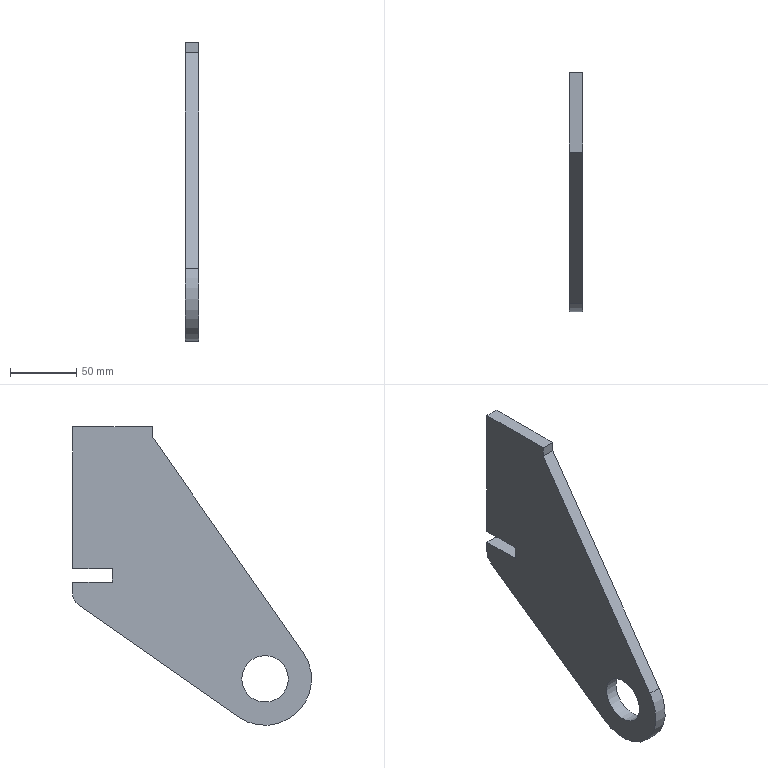Part | STEP file | subframe cylinder mounting plate--000.001--20240928 | 1 solid | 14 faces | box 10 x 180 x 225 mm | volume 214706 mm3 | plane 11 | cylinder 3 | commonest cylinder face diameters 20 x1 35 x1 70 x1
STEP:
#1=CARTESIAN_POINT('',(0.,0.,0.));
#2=DIRECTION('',(0.,0.,1.));
#3=DIRECTION('',(1.,0.,0.));
#4=AXIS2_PLACEMENT_3D('',#1,#2,#3);
#5=CARTESIAN_POINT('',(-10.,145.,64.009));
#6=VERTEX_POINT('',#5);
#7=CARTESIAN_POINT('',(-10.,145.,73.));
#8=VERTEX_POINT('',#7);
#9=CARTESIAN_POINT('',(-10.,145.,-567.));
#10=DIRECTION('',(0.,0.,1.));
#11=VECTOR('',#10,1.);
#12=LINE('',#9,#11);
#13=CARTESIAN_POINT('',(1830.173,145.,190.));
#14=DIRECTION('',(0.,-1.,0.));
#15=DIRECTION('',(1.,0.,0.));
#16=AXIS2_PLACEMENT_3D('',#13,#14,#15);
#17=PLANE('',#16);
#18=CARTESIAN_POINT('',(-1840.173,-757.));
#19=DIRECTION('',(0.,1.));
#20=VECTOR('',#19,1.);
#21=LINE('',#18,#20);
#22=(GEOMETRIC_REPRESENTATION_CONTEXT(2)PARAMETRIC_REPRESENTATION_CONTEXT()REPRESENTATION_CONTEXT('',''));
#23=DEFINITIONAL_REPRESENTATION('',(#21),#22);
#24=PCURVE('',#17,#23);
#25=CARTESIAN_POINT('',(-10.,145.,-567.));
#26=DIRECTION('',(1.,0.,0.));
#27=DIRECTION('',(0.,1.,0.));
#28=AXIS2_PLACEMENT_3D('',#25,#26,#27);
#29=PLANE('',#28);
#30=CARTESIAN_POINT('',(0.,0.));
#31=DIRECTION('',(0.,1.));
#32=VECTOR('',#31,1.);
#33=LINE('',#30,#32);
#34=(GEOMETRIC_REPRESENTATION_CONTEXT(2)PARAMETRIC_REPRESENTATION_CONTEXT()REPRESENTATION_CONTEXT('',''));
#35=DEFINITIONAL_REPRESENTATION('',(#33),#34);
#36=PCURVE('',#29,#35);
#37=SURFACE_CURVE('',#12,(#24,#36),.PCURVE_S1.);
#38=EDGE_CURVE('',#6,#8,#37,.T.);
#39=ORIENTED_EDGE('',*,*,#38,.T.);
#40=CARTESIAN_POINT('',(0.,145.,73.));
#41=VERTEX_POINT('',#40);
#42=CARTESIAN_POINT('',(100.,145.,73.));
#43=DIRECTION('',(1.,0.,0.));
#44=VECTOR('',#43,1.);
#45=LINE('',#42,#44);
#46=CARTESIAN_POINT('',(-1730.173,-117.));
#47=DIRECTION('',(1.,0.));
#48=VECTOR('',#47,1.);
#49=LINE('',#46,#48);
#50=(GEOMETRIC_REPRESENTATION_CONTEXT(2)PARAMETRIC_REPRESENTATION_CONTEXT()REPRESENTATION_CONTEXT('',''));
#51=DEFINITIONAL_REPRESENTATION('',(#49),#50);
#52=PCURVE('',#17,#51);
#53=CARTESIAN_POINT('',(100.,85.,73.));
#54=DIRECTION('',(0.,0.,1.));
#55=DIRECTION('',(0.,-1.,0.));
#56=AXIS2_PLACEMENT_3D('',#53,#54,#55);
#57=PLANE('',#56);
#58=CARTESIAN_POINT('',(-60.,0.));
#59=DIRECTION('',(0.,1.));
#60=VECTOR('',#59,1.);
#61=LINE('',#58,#60);
#62=(GEOMETRIC_REPRESENTATION_CONTEXT(2)PARAMETRIC_REPRESENTATION_CONTEXT()REPRESENTATION_CONTEXT('',''));
#63=DEFINITIONAL_REPRESENTATION('',(#61),#62);
#64=PCURVE('',#57,#63);
#65=SURFACE_CURVE('',#45,(#52,#64),.PCURVE_S1.);
#66=EDGE_CURVE('',#8,#41,#65,.T.);
#67=ORIENTED_EDGE('',*,*,#66,.T.);
#68=CARTESIAN_POINT('',(0.,145.,64.009));
#69=VERTEX_POINT('',#68);
#70=CARTESIAN_POINT('',(0.,145.,-567.));
#71=DIRECTION('',(0.,0.,1.));
#72=VECTOR('',#71,1.);
#73=LINE('',#70,#72);
#74=CARTESIAN_POINT('',(-1830.173,-757.));
#75=DIRECTION('',(0.,1.));
#76=VECTOR('',#75,1.);
#77=LINE('',#74,#76);
#78=(GEOMETRIC_REPRESENTATION_CONTEXT(2)PARAMETRIC_REPRESENTATION_CONTEXT()REPRESENTATION_CONTEXT('',''));
#79=DEFINITIONAL_REPRESENTATION('',(#77),#78);
#80=PCURVE('',#17,#79);
#81=CARTESIAN_POINT('',(0.,145.,-567.));
#82=DIRECTION('',(1.,0.,0.));
#83=DIRECTION('',(0.,1.,0.));
#84=AXIS2_PLACEMENT_3D('',#81,#82,#83);
#85=PLANE('',#84);
#86=CARTESIAN_POINT('',(0.,0.));
#87=DIRECTION('',(0.,1.));
#88=VECTOR('',#87,1.);
#89=LINE('',#86,#88);
#90=(GEOMETRIC_REPRESENTATION_CONTEXT(2)PARAMETRIC_REPRESENTATION_CONTEXT()REPRESENTATION_CONTEXT('',''));
#91=DEFINITIONAL_REPRESENTATION('',(#89),#90);
#92=PCURVE('',#85,#91);
#93=SURFACE_CURVE('',#73,(#80,#92),.PCURVE_S1.);
#94=EDGE_CURVE('',#69,#41,#93,.T.);
#95=ORIENTED_EDGE('',*,*,#94,.F.);
#96=CARTESIAN_POINT('',(1830.173,145.,64.009));
#97=DIRECTION('',(-1.,0.,0.));
#98=VECTOR('',#97,1.);
#99=LINE('',#96,#98);
#100=CARTESIAN_POINT('',(0.,-125.991));
#101=DIRECTION('',(-1.,0.));
#102=VECTOR('',#101,1.);
#103=LINE('',#100,#102);
#104=(GEOMETRIC_REPRESENTATION_CONTEXT(2)PARAMETRIC_REPRESENTATION_CONTEXT()REPRESENTATION_CONTEXT('',''));
#105=DEFINITIONAL_REPRESENTATION('',(#103),#104);
#106=PCURVE('',#17,#105);
#107=CARTESIAN_POINT('',(250.,135.,64.009));
#108=DIRECTION('',(-1.,0.,0.));
#109=DIRECTION('',(0.,1.,0.));
#110=AXIS2_PLACEMENT_3D('',#107,#108,#109);
#111=CYLINDRICAL_SURFACE('',#110,10.);
#112=CARTESIAN_POINT('',(0.,-1580.173));
#113=DIRECTION('',(0.,1.));
#114=VECTOR('',#113,1.);
#115=LINE('',#112,#114);
#116=(GEOMETRIC_REPRESENTATION_CONTEXT(2)PARAMETRIC_REPRESENTATION_CONTEXT()REPRESENTATION_CONTEXT('',''));
#117=DEFINITIONAL_REPRESENTATION('',(#115),#116);
#118=PCURVE('',#111,#117);
#119=SURFACE_CURVE('',#99,(#106,#118),.PCURVE_S1.);
#120=EDGE_CURVE('',#69,#6,#119,.T.);
#121=ORIENTED_EDGE('',*,*,#120,.T.);
#122=EDGE_LOOP('',(#39,#67,#95,#121));
#123=FACE_BOUND('',#122,.T.);
#124=ADVANCED_FACE('',(#123),#17,.F.);
#125=CARTESIAN_POINT('',(-10.,145.,83.));
#126=VERTEX_POINT('',#125);
#127=CARTESIAN_POINT('',(0.,145.,83.));
#128=VERTEX_POINT('',#127);
#129=CARTESIAN_POINT('',(100.,145.,83.));
#130=DIRECTION('',(1.,0.,0.));
#131=VECTOR('',#130,1.);
#132=LINE('',#129,#131);
#133=CARTESIAN_POINT('',(1830.173,145.,190.));
#134=DIRECTION('',(0.,-1.,0.));
#135=DIRECTION('',(1.,0.,0.));
#136=AXIS2_PLACEMENT_3D('',#133,#134,#135);
#137=PLANE('',#136);
#138=CARTESIAN_POINT('',(-1730.173,-107.));
#139=DIRECTION('',(1.,0.));
#140=VECTOR('',#139,1.);
#141=LINE('',#138,#140);
#142=(GEOMETRIC_REPRESENTATION_CONTEXT(2)PARAMETRIC_REPRESENTATION_CONTEXT()REPRESENTATION_CONTEXT('',''));
#143=DEFINITIONAL_REPRESENTATION('',(#141),#142);
#144=PCURVE('',#137,#143);
#145=CARTESIAN_POINT('',(100.,85.,83.));
#146=DIRECTION('',(0.,0.,1.));
#147=DIRECTION('',(0.,-1.,0.));
#148=AXIS2_PLACEMENT_3D('',#145,#146,#147);
#149=PLANE('',#148);
#150=CARTESIAN_POINT('',(-60.,0.));
#151=DIRECTION('',(0.,1.));
#152=VECTOR('',#151,1.);
#153=LINE('',#150,#152);
#154=(GEOMETRIC_REPRESENTATION_CONTEXT(2)PARAMETRIC_REPRESENTATION_CONTEXT()REPRESENTATION_CONTEXT('',''));
#155=DEFINITIONAL_REPRESENTATION('',(#153),#154);
#156=PCURVE('',#149,#155);
#157=SURFACE_CURVE('',#132,(#144,#156),.PCURVE_S1.);
#158=EDGE_CURVE('',#126,#128,#157,.T.);
#159=ORIENTED_EDGE('',*,*,#158,.F.);
#160=CARTESIAN_POINT('',(-10.,145.,190.));
#161=VERTEX_POINT('',#160);
#162=CARTESIAN_POINT('',(-10.,145.,-567.));
#163=DIRECTION('',(0.,0.,1.));
#164=VECTOR('',#163,1.);
#165=LINE('',#162,#164);
#166=CARTESIAN_POINT('',(-1840.173,-757.));
#167=DIRECTION('',(0.,1.));
#168=VECTOR('',#167,1.);
#169=LINE('',#166,#168);
#170=(GEOMETRIC_REPRESENTATION_CONTEXT(2)PARAMETRIC_REPRESENTATION_CONTEXT()REPRESENTATION_CONTEXT('',''));
#171=DEFINITIONAL_REPRESENTATION('',(#169),#170);
#172=PCURVE('',#137,#171);
#173=CARTESIAN_POINT('',(0.,0.));
#174=DIRECTION('',(0.,1.));
#175=VECTOR('',#174,1.);
#176=LINE('',#173,#175);
#177=(GEOMETRIC_REPRESENTATION_CONTEXT(2)PARAMETRIC_REPRESENTATION_CONTEXT()REPRESENTATION_CONTEXT('',''));
#178=DEFINITIONAL_REPRESENTATION('',(#176),#177);
#179=PCURVE('',#29,#178);
#180=SURFACE_CURVE('',#165,(#172,#179),.PCURVE_S1.);
#181=EDGE_CURVE('',#126,#161,#180,.T.);
#182=ORIENTED_EDGE('',*,*,#181,.T.);
#183=CARTESIAN_POINT('',(0.,145.,190.));
#184=VERTEX_POINT('',#183);
#185=CARTESIAN_POINT('',(1830.173,145.,190.));
#186=DIRECTION('',(1.,0.,0.));
#187=VECTOR('',#186,1.);
#188=LINE('',#185,#187);
#189=CARTESIAN_POINT('',(0.,0.));
#190=DIRECTION('',(1.,0.));
#191=VECTOR('',#190,1.);
#192=LINE('',#189,#191);
#193=(GEOMETRIC_REPRESENTATION_CONTEXT(2)PARAMETRIC_REPRESENTATION_CONTEXT()REPRESENTATION_CONTEXT('',''));
#194=DEFINITIONAL_REPRESENTATION('',(#192),#193);
#195=PCURVE('',#137,#194);
#196=CARTESIAN_POINT('',(250.,115.,190.));
#197=DIRECTION('',(0.,0.,1.));
#198=DIRECTION('',(-0.2756,0.9613,0.));
#199=AXIS2_PLACEMENT_3D('',#196,#197,#198);
#200=PLANE('',#199);
#201=CARTESIAN_POINT('',(-406.717,-1527.229));
#202=DIRECTION('',(-0.2756,-0.9613));
#203=VECTOR('',#202,1.);
#204=LINE('',#201,#203);
#205=(GEOMETRIC_REPRESENTATION_CONTEXT(2)PARAMETRIC_REPRESENTATION_CONTEXT()REPRESENTATION_CONTEXT('',''));
#206=DEFINITIONAL_REPRESENTATION('',(#204),#205);
#207=PCURVE('',#200,#206);
#208=SURFACE_CURVE('',#188,(#195,#207),.PCURVE_S1.);
#209=EDGE_CURVE('',#161,#184,#208,.T.);
#210=ORIENTED_EDGE('',*,*,#209,.T.);
#211=CARTESIAN_POINT('',(0.,145.,-567.));
#212=DIRECTION('',(0.,0.,1.));
#213=VECTOR('',#212,1.);
#214=LINE('',#211,#213);
#215=CARTESIAN_POINT('',(-1830.173,-757.));
#216=DIRECTION('',(0.,1.));
#217=VECTOR('',#216,1.);
#218=LINE('',#215,#217);
#219=(GEOMETRIC_REPRESENTATION_CONTEXT(2)PARAMETRIC_REPRESENTATION_CONTEXT()REPRESENTATION_CONTEXT('',''));
#220=DEFINITIONAL_REPRESENTATION('',(#218),#219);
#221=PCURVE('',#137,#220);
#222=CARTESIAN_POINT('',(0.,0.));
#223=DIRECTION('',(0.,1.));
#224=VECTOR('',#223,1.);
#225=LINE('',#222,#224);
#226=(GEOMETRIC_REPRESENTATION_CONTEXT(2)PARAMETRIC_REPRESENTATION_CONTEXT()REPRESENTATION_CONTEXT('',''));
#227=DEFINITIONAL_REPRESENTATION('',(#225),#226);
#228=PCURVE('',#85,#227);
#229=SURFACE_CURVE('',#214,(#221,#228),.PCURVE_S1.);
#230=EDGE_CURVE('',#128,#184,#229,.T.);
#231=ORIENTED_EDGE('',*,*,#230,.F.);
#232=EDGE_LOOP('',(#159,#182,#210,#231));
#233=FACE_BOUND('',#232,.T.);
#234=ADVANCED_FACE('',(#233),#137,.F.);
#235=CARTESIAN_POINT('',(-10.,115.,83.));
#236=VERTEX_POINT('',#235);
#237=CARTESIAN_POINT('',(-10.,145.,83.));
#238=DIRECTION('',(0.,-1.,0.));
#239=VECTOR('',#238,1.);
#240=LINE('',#237,#239);
#241=CARTESIAN_POINT('',(0.,650.));
#242=DIRECTION('',(-1.,0.));
#243=VECTOR('',#242,1.);
#244=LINE('',#241,#243);
#245=(GEOMETRIC_REPRESENTATION_CONTEXT(2)PARAMETRIC_REPRESENTATION_CONTEXT()REPRESENTATION_CONTEXT('',''));
#246=DEFINITIONAL_REPRESENTATION('',(#244),#245);
#247=PCURVE('',#29,#246);
#248=CARTESIAN_POINT('',(-60.,-110.));
#249=DIRECTION('',(1.,0.));
#250=VECTOR('',#249,1.);
#251=LINE('',#248,#250);
#252=(GEOMETRIC_REPRESENTATION_CONTEXT(2)PARAMETRIC_REPRESENTATION_CONTEXT()REPRESENTATION_CONTEXT('',''));
#253=DEFINITIONAL_REPRESENTATION('',(#251),#252);
#254=PCURVE('',#149,#253);
#255=SURFACE_CURVE('',#240,(#247,#254),.PCURVE_S1.);
#256=EDGE_CURVE('',#126,#236,#255,.T.);
#257=ORIENTED_EDGE('',*,*,#256,.T.);
#258=CARTESIAN_POINT('',(-10.,115.,73.));
#259=VERTEX_POINT('',#258);
#260=CARTESIAN_POINT('',(-10.,115.,78.));
#261=DIRECTION('',(0.,0.,-1.));
#262=VECTOR('',#261,1.);
#263=LINE('',#260,#262);
#264=CARTESIAN_POINT('',(-30.,645.));
#265=DIRECTION('',(0.,-1.));
#266=VECTOR('',#265,1.);
#267=LINE('',#264,#266);
#268=(GEOMETRIC_REPRESENTATION_CONTEXT(2)PARAMETRIC_REPRESENTATION_CONTEXT()REPRESENTATION_CONTEXT('',''));
#269=DEFINITIONAL_REPRESENTATION('',(#267),#268);
#270=PCURVE('',#29,#269);
#271=CARTESIAN_POINT('',(95.,115.,78.));
#272=DIRECTION('',(0.,1.,0.));
#273=DIRECTION('',(1.,0.,0.));
#274=AXIS2_PLACEMENT_3D('',#271,#272,#273);
#275=PLANE('',#274);
#276=CARTESIAN_POINT('',(-105.,0.));
#277=DIRECTION('',(0.,1.));
#278=VECTOR('',#277,1.);
#279=LINE('',#276,#278);
#280=(GEOMETRIC_REPRESENTATION_CONTEXT(2)PARAMETRIC_REPRESENTATION_CONTEXT()REPRESENTATION_CONTEXT('',''));
#281=DEFINITIONAL_REPRESENTATION('',(#279),#280);
#282=PCURVE('',#275,#281);
#283=SURFACE_CURVE('',#263,(#270,#282),.PCURVE_S1.);
#284=EDGE_CURVE('',#236,#259,#283,.T.);
#285=ORIENTED_EDGE('',*,*,#284,.T.);
#286=CARTESIAN_POINT('',(-10.,145.,73.));
#287=DIRECTION('',(0.,1.,0.));
#288=VECTOR('',#287,1.);
#289=LINE('',#286,#288);
#290=CARTESIAN_POINT('',(0.,640.));
#291=DIRECTION('',(1.,0.));
#292=VECTOR('',#291,1.);
#293=LINE('',#290,#292);
#294=(GEOMETRIC_REPRESENTATION_CONTEXT(2)PARAMETRIC_REPRESENTATION_CONTEXT()REPRESENTATION_CONTEXT('',''));
#295=DEFINITIONAL_REPRESENTATION('',(#293),#294);
#296=PCURVE('',#29,#295);
#297=CARTESIAN_POINT('',(-60.,-110.));
#298=DIRECTION('',(-1.,0.));
#299=VECTOR('',#298,1.);
#300=LINE('',#297,#299);
#301=(GEOMETRIC_REPRESENTATION_CONTEXT(2)PARAMETRIC_REPRESENTATION_CONTEXT()REPRESENTATION_CONTEXT('',''));
#302=DEFINITIONAL_REPRESENTATION('',(#300),#301);
#303=PCURVE('',#57,#302);
#304=SURFACE_CURVE('',#289,(#296,#303),.PCURVE_S1.);
#305=EDGE_CURVE('',#259,#8,#304,.T.);
#306=ORIENTED_EDGE('',*,*,#305,.T.);
#307=ORIENTED_EDGE('',*,*,#38,.F.);
#308=CARTESIAN_POINT('',(-10.,140.736,55.817));
#309=VERTEX_POINT('',#308);
#310=CARTESIAN_POINT('',(-10.,135.,64.009));
#311=DIRECTION('',(-1.,0.,0.));
#312=DIRECTION('',(0.,0.,-1.));
#313=AXIS2_PLACEMENT_3D('',#310,#311,#312);
#314=CIRCLE('',#313,10.);
#315=CARTESIAN_POINT('',(-10.,621.009));
#316=CARTESIAN_POINT('',(-27.321,621.009));
#317=CARTESIAN_POINT('',(-18.66,636.009));
#318=CARTESIAN_POINT('',(-10.,651.009));
#319=CARTESIAN_POINT('',(-1.34,636.009));
#320=CARTESIAN_POINT('',(7.321,621.009));
#321=CARTESIAN_POINT('',(-10.,621.009));
#322=(BOUNDED_CURVE()B_SPLINE_CURVE(2,(#315,#316,#317,#318,#319,#320,#321),.UNSPECIFIED.,.T.,.F.)B_SPLINE_CURVE_WITH_KNOTS((1,2,2,2,2,1),(-2.094,0.,2.094,4.189,6.283,8.378),.UNSPECIFIED.)CURVE()GEOMETRIC_REPRESENTATION_ITEM()RATIONAL_B_SPLINE_CURVE((1.,0.5,1.,0.5,1.,0.5,1.))REPRESENTATION_ITEM(''));
#323=(GEOMETRIC_REPRESENTATION_CONTEXT(2)PARAMETRIC_REPRESENTATION_CONTEXT()REPRESENTATION_CONTEXT('',''));
#324=DEFINITIONAL_REPRESENTATION('',(#322),#323);
#325=PCURVE('',#29,#324);
#326=CARTESIAN_POINT('',(-4.712,260.));
#327=DIRECTION('',(1.,0.));
#328=VECTOR('',#327,1.);
#329=LINE('',#326,#328);
#330=(GEOMETRIC_REPRESENTATION_CONTEXT(2)PARAMETRIC_REPRESENTATION_CONTEXT()REPRESENTATION_CONTEXT('',''));
#331=DEFINITIONAL_REPRESENTATION('',(#329),#330);
#332=PCURVE('',#111,#331);
#333=SURFACE_CURVE('',#314,(#325,#332),.PCURVE_S1.);
#334=EDGE_CURVE('',#6,#309,#333,.T.);
#335=ORIENTED_EDGE('',*,*,#334,.T.);
#336=CARTESIAN_POINT('',(-10.,20.075,-28.67));
#337=VERTEX_POINT('',#336);
#338=CARTESIAN_POINT('',(-10.,-149.031,-147.08));
#339=DIRECTION('',(0.,-0.8192,-0.5736));
#340=VECTOR('',#339,1.);
#341=LINE('',#338,#340);
#342=CARTESIAN_POINT('',(-294.031,419.92));
#343=DIRECTION('',(-0.8192,-0.5736));
#344=VECTOR('',#343,1.);
#345=LINE('',#342,#344);
#346=(GEOMETRIC_REPRESENTATION_CONTEXT(2)PARAMETRIC_REPRESENTATION_CONTEXT()REPRESENTATION_CONTEXT('',''));
#347=DEFINITIONAL_REPRESENTATION('',(#345),#346);
#348=PCURVE('',#29,#347);
#349=CARTESIAN_POINT('',(250.,114.278,37.291));
#350=DIRECTION('',(0.,0.5736,-0.8192));
#351=DIRECTION('',(0.2756,-0.7874,-0.5514));
#352=AXIS2_PLACEMENT_3D('',#349,#350,#351);
#353=PLANE('',#352);
#354=CARTESIAN_POINT('',(237.323,338.529));
#355=DIRECTION('',(0.9613,0.2756));
#356=VECTOR('',#355,1.);
#357=LINE('',#354,#356);
#358=(GEOMETRIC_REPRESENTATION_CONTEXT(2)PARAMETRIC_REPRESENTATION_CONTEXT()REPRESENTATION_CONTEXT('',''));
#359=DEFINITIONAL_REPRESENTATION('',(#357),#358);
#360=PCURVE('',#353,#359);
#361=SURFACE_CURVE('',#341,(#348,#360),.PCURVE_S1.);
#362=EDGE_CURVE('',#309,#337,#361,.T.);
#363=ORIENTED_EDGE('',*,*,#362,.T.);
#364=CARTESIAN_POINT('',(-10.,-28.67,20.075));
#365=VERTEX_POINT('',#364);
#366=CARTESIAN_POINT('',(-10.,0.,0.));
#367=DIRECTION('',(-1.,0.,0.));
#368=DIRECTION('',(0.,0.,-1.));
#369=AXIS2_PLACEMENT_3D('',#366,#367,#368);
#370=CIRCLE('',#369,35.);
#371=CARTESIAN_POINT('',(-145.,532.));
#372=CARTESIAN_POINT('',(-205.622,532.));
#373=CARTESIAN_POINT('',(-175.311,584.5));
#374=CARTESIAN_POINT('',(-145.,637.));
#375=CARTESIAN_POINT('',(-114.689,584.5));
#376=CARTESIAN_POINT('',(-84.378,532.));
#377=CARTESIAN_POINT('',(-145.,532.));
#378=(BOUNDED_CURVE()B_SPLINE_CURVE(2,(#371,#372,#373,#374,#375,#376,#377),.UNSPECIFIED.,.T.,.F.)B_SPLINE_CURVE_WITH_KNOTS((1,2,2,2,2,1),(-2.094,0.,2.094,4.189,6.283,8.378),.UNSPECIFIED.)CURVE()GEOMETRIC_REPRESENTATION_ITEM()RATIONAL_B_SPLINE_CURVE((1.,0.5,1.,0.5,1.,0.5,1.))REPRESENTATION_ITEM(''));
#379=(GEOMETRIC_REPRESENTATION_CONTEXT(2)PARAMETRIC_REPRESENTATION_CONTEXT()REPRESENTATION_CONTEXT('',''));
#380=DEFINITIONAL_REPRESENTATION('',(#378),#379);
#381=PCURVE('',#29,#380);
#382=CARTESIAN_POINT('',(-30.,0.,0.));
#383=DIRECTION('',(1.,0.,0.));
#384=DIRECTION('',(0.,0.,1.));
#385=AXIS2_PLACEMENT_3D('',#382,#383,#384);
#386=CYLINDRICAL_SURFACE('',#385,35.);
#387=CARTESIAN_POINT('',(9.425,20.));
#388=DIRECTION('',(-1.,0.));
#389=VECTOR('',#388,1.);
#390=LINE('',#387,#389);
#391=(GEOMETRIC_REPRESENTATION_CONTEXT(2)PARAMETRIC_REPRESENTATION_CONTEXT()REPRESENTATION_CONTEXT('',''));
#392=DEFINITIONAL_REPRESENTATION('',(#390),#391);
#393=PCURVE('',#386,#392);
#394=SURFACE_CURVE('',#370,(#381,#393),.PCURVE_S1.);
#395=EDGE_CURVE('',#337,#365,#394,.T.);
#396=ORIENTED_EDGE('',*,*,#395,.T.);
#397=CARTESIAN_POINT('',(-10.,85.,182.413));
#398=VERTEX_POINT('',#397);
#399=CARTESIAN_POINT('',(-10.,-25.831,24.13));
#400=DIRECTION('',(0.,0.5736,0.8192));
#401=VECTOR('',#400,1.);
#402=LINE('',#399,#401);
#403=CARTESIAN_POINT('',(-170.831,591.13));
#404=DIRECTION('',(0.5736,0.8192));
#405=VECTOR('',#404,1.);
#406=LINE('',#403,#405);
#407=(GEOMETRIC_REPRESENTATION_CONTEXT(2)PARAMETRIC_REPRESENTATION_CONTEXT()REPRESENTATION_CONTEXT('',''));
#408=DEFINITIONAL_REPRESENTATION('',(#406),#407);
#409=PCURVE('',#29,#408);
#410=CARTESIAN_POINT('',(-30.,-25.831,24.13));
#411=DIRECTION('',(0.,-0.8192,0.5736));
#412=DIRECTION('',(-1.,0.,0.));
#413=AXIS2_PLACEMENT_3D('',#410,#411,#412);
#414=PLANE('',#413);
#415=CARTESIAN_POINT('',(-20.,0.));
#416=DIRECTION('',(0.,-1.));
#417=VECTOR('',#416,1.);
#418=LINE('',#415,#417);
#419=(GEOMETRIC_REPRESENTATION_CONTEXT(2)PARAMETRIC_REPRESENTATION_CONTEXT()REPRESENTATION_CONTEXT('',''));
#420=DEFINITIONAL_REPRESENTATION('',(#418),#419);
#421=PCURVE('',#414,#420);
#422=SURFACE_CURVE('',#402,(#409,#421),.PCURVE_S1.);
#423=EDGE_CURVE('',#365,#398,#422,.T.);
#424=ORIENTED_EDGE('',*,*,#423,.T.);
#425=CARTESIAN_POINT('',(-10.,85.,190.));
#426=VERTEX_POINT('',#425);
#427=CARTESIAN_POINT('',(-10.,85.,-567.));
#428=DIRECTION('',(0.,0.,1.));
#429=VECTOR('',#428,1.);
#430=LINE('',#427,#429);
#431=CARTESIAN_POINT('',(-60.,0.));
#432=DIRECTION('',(0.,1.));
#433=VECTOR('',#432,1.);
#434=LINE('',#431,#433);
#435=(GEOMETRIC_REPRESENTATION_CONTEXT(2)PARAMETRIC_REPRESENTATION_CONTEXT()REPRESENTATION_CONTEXT('',''));
#436=DEFINITIONAL_REPRESENTATION('',(#434),#435);
#437=PCURVE('',#29,#436);
#438=CARTESIAN_POINT('',(-5.,85.,210.));
#439=DIRECTION('',(0.,1.,0.));
#440=DIRECTION('',(0.,0.,-1.));
#441=AXIS2_PLACEMENT_3D('',#438,#439,#440);
#442=PLANE('',#441);
#443=CARTESIAN_POINT('',(777.,5.));
#444=DIRECTION('',(-1.,0.));
#445=VECTOR('',#444,1.);
#446=LINE('',#443,#445);
#447=(GEOMETRIC_REPRESENTATION_CONTEXT(2)PARAMETRIC_REPRESENTATION_CONTEXT()REPRESENTATION_CONTEXT('',''));
#448=DEFINITIONAL_REPRESENTATION('',(#446),#447);
#449=PCURVE('',#442,#448);
#450=SURFACE_CURVE('',#430,(#437,#449),.PCURVE_S1.);
#451=EDGE_CURVE('',#398,#426,#450,.T.);
#452=ORIENTED_EDGE('',*,*,#451,.T.);
#453=CARTESIAN_POINT('',(-10.,145.,190.));
#454=DIRECTION('',(0.,-1.,0.));
#455=VECTOR('',#454,1.);
#456=LINE('',#453,#455);
#457=CARTESIAN_POINT('',(0.,757.));
#458=DIRECTION('',(-1.,0.));
#459=VECTOR('',#458,1.);
#460=LINE('',#457,#459);
#461=(GEOMETRIC_REPRESENTATION_CONTEXT(2)PARAMETRIC_REPRESENTATION_CONTEXT()REPRESENTATION_CONTEXT('',''));
#462=DEFINITIONAL_REPRESENTATION('',(#460),#461);
#463=PCURVE('',#29,#462);
#464=CARTESIAN_POINT('',(100.504,241.659));
#465=DIRECTION('',(-0.9613,0.2756));
#466=VECTOR('',#465,1.);
#467=LINE('',#464,#466);
#468=(GEOMETRIC_REPRESENTATION_CONTEXT(2)PARAMETRIC_REPRESENTATION_CONTEXT()REPRESENTATION_CONTEXT('',''));
#469=DEFINITIONAL_REPRESENTATION('',(#467),#468);
#470=PCURVE('',#200,#469);
#471=SURFACE_CURVE('',#456,(#463,#470),.PCURVE_S1.);
#472=EDGE_CURVE('',#161,#426,#471,.T.);
#473=ORIENTED_EDGE('',*,*,#472,.F.);
#474=ORIENTED_EDGE('',*,*,#181,.F.);
#475=EDGE_LOOP('',(#257,#285,#306,#307,#335,#363,#396,#424,#452,#473,#474));
#476=FACE_BOUND('',#475,.T.);
#477=CARTESIAN_POINT('',(-10.,-17.5,0.));
#478=VERTEX_POINT('',#477);
#479=CARTESIAN_POINT('',(-10.,0.,0.));
#480=DIRECTION('',(1.,0.,0.));
#481=DIRECTION('',(0.,-1.,0.));
#482=AXIS2_PLACEMENT_3D('',#479,#480,#481);
#483=CIRCLE('',#482,17.5);
#484=CARTESIAN_POINT('',(-145.,567.));
#485=DIRECTION('',(-1.,0.));
#486=AXIS2_PLACEMENT_2D('',#484,#485);
#487=CIRCLE('',#486,17.5);
#488=(GEOMETRIC_REPRESENTATION_CONTEXT(2)PARAMETRIC_REPRESENTATION_CONTEXT()REPRESENTATION_CONTEXT('',''));
#489=DEFINITIONAL_REPRESENTATION('',(#487),#488);
#490=PCURVE('',#29,#489);
#491=CARTESIAN_POINT('',(-360.,0.,0.));
#492=DIRECTION('',(1.,0.,0.));
#493=DIRECTION('',(0.,1.,0.));
#494=AXIS2_PLACEMENT_3D('',#491,#492,#493);
#495=CYLINDRICAL_SURFACE('',#494,17.5);
#496=CARTESIAN_POINT('',(3.142,350.));
#497=DIRECTION('',(1.,0.));
#498=VECTOR('',#497,1.);
#499=LINE('',#496,#498);
#500=(GEOMETRIC_REPRESENTATION_CONTEXT(2)PARAMETRIC_REPRESENTATION_CONTEXT()REPRESENTATION_CONTEXT('',''));
#501=DEFINITIONAL_REPRESENTATION('',(#499),#500);
#502=PCURVE('',#495,#501);
#503=SURFACE_CURVE('',#483,(#490,#502),.PCURVE_S1.);
#504=EDGE_CURVE('',#478,#478,#503,.T.);
#505=ORIENTED_EDGE('',*,*,#504,.T.);
#506=EDGE_LOOP('',(#505));
#507=FACE_BOUND('',#506,.T.);
#508=ADVANCED_FACE('',(#476,#507),#29,.F.);
#509=CARTESIAN_POINT('',(0.,115.,83.));
#510=VERTEX_POINT('',#509);
#511=CARTESIAN_POINT('',(0.,115.,73.));
#512=VERTEX_POINT('',#511);
#513=CARTESIAN_POINT('',(0.,115.,78.));
#514=DIRECTION('',(0.,0.,-1.));
#515=VECTOR('',#514,1.);
#516=LINE('',#513,#515);
#517=CARTESIAN_POINT('',(-30.,645.));
#518=DIRECTION('',(0.,-1.));
#519=VECTOR('',#518,1.);
#520=LINE('',#517,#519);
#521=(GEOMETRIC_REPRESENTATION_CONTEXT(2)PARAMETRIC_REPRESENTATION_CONTEXT()REPRESENTATION_CONTEXT('',''));
#522=DEFINITIONAL_REPRESENTATION('',(#520),#521);
#523=PCURVE('',#85,#522);
#524=CARTESIAN_POINT('',(-95.,0.));
#525=DIRECTION('',(0.,1.));
#526=VECTOR('',#525,1.);
#527=LINE('',#524,#526);
#528=(GEOMETRIC_REPRESENTATION_CONTEXT(2)PARAMETRIC_REPRESENTATION_CONTEXT()REPRESENTATION_CONTEXT('',''));
#529=DEFINITIONAL_REPRESENTATION('',(#527),#528);
#530=PCURVE('',#275,#529);
#531=SURFACE_CURVE('',#516,(#523,#530),.PCURVE_S1.);
#532=EDGE_CURVE('',#510,#512,#531,.T.);
#533=ORIENTED_EDGE('',*,*,#532,.F.);
#534=CARTESIAN_POINT('',(0.,145.,83.));
#535=DIRECTION('',(0.,-1.,0.));
#536=VECTOR('',#535,1.);
#537=LINE('',#534,#536);
#538=CARTESIAN_POINT('',(0.,650.));
#539=DIRECTION('',(-1.,0.));
#540=VECTOR('',#539,1.);
#541=LINE('',#538,#540);
#542=(GEOMETRIC_REPRESENTATION_CONTEXT(2)PARAMETRIC_REPRESENTATION_CONTEXT()REPRESENTATION_CONTEXT('',''));
#543=DEFINITIONAL_REPRESENTATION('',(#541),#542);
#544=PCURVE('',#85,#543);
#545=CARTESIAN_POINT('',(-60.,-100.));
#546=DIRECTION('',(1.,0.));
#547=VECTOR('',#546,1.);
#548=LINE('',#545,#547);
#549=(GEOMETRIC_REPRESENTATION_CONTEXT(2)PARAMETRIC_REPRESENTATION_CONTEXT()REPRESENTATION_CONTEXT('',''));
#550=DEFINITIONAL_REPRESENTATION('',(#548),#549);
#551=PCURVE('',#149,#550);
#552=SURFACE_CURVE('',#537,(#544,#551),.PCURVE_S1.);
#553=EDGE_CURVE('',#128,#510,#552,.T.);
#554=ORIENTED_EDGE('',*,*,#553,.F.);
#555=ORIENTED_EDGE('',*,*,#230,.T.);
#556=CARTESIAN_POINT('',(0.,85.,190.));
#557=VERTEX_POINT('',#556);
#558=CARTESIAN_POINT('',(0.,145.,190.));
#559=DIRECTION('',(0.,-1.,0.));
#560=VECTOR('',#559,1.);
#561=LINE('',#558,#560);
#562=CARTESIAN_POINT('',(0.,757.));
#563=DIRECTION('',(-1.,0.));
#564=VECTOR('',#563,1.);
#565=LINE('',#562,#564);
#566=(GEOMETRIC_REPRESENTATION_CONTEXT(2)PARAMETRIC_REPRESENTATION_CONTEXT()REPRESENTATION_CONTEXT('',''));
#567=DEFINITIONAL_REPRESENTATION('',(#565),#566);
#568=PCURVE('',#85,#567);
#569=CARTESIAN_POINT('',(97.747,232.046));
#570=DIRECTION('',(-0.9613,0.2756));
#571=VECTOR('',#570,1.);
#572=LINE('',#569,#571);
#573=(GEOMETRIC_REPRESENTATION_CONTEXT(2)PARAMETRIC_REPRESENTATION_CONTEXT()REPRESENTATION_CONTEXT('',''));
#574=DEFINITIONAL_REPRESENTATION('',(#572),#573);
#575=PCURVE('',#200,#574);
#576=SURFACE_CURVE('',#561,(#568,#575),.PCURVE_S1.);
#577=EDGE_CURVE('',#184,#557,#576,.T.);
#578=ORIENTED_EDGE('',*,*,#577,.T.);
#579=CARTESIAN_POINT('',(0.,85.,182.413));
#580=VERTEX_POINT('',#579);
#581=CARTESIAN_POINT('',(0.,85.,-567.));
#582=DIRECTION('',(0.,0.,1.));
#583=VECTOR('',#582,1.);
#584=LINE('',#581,#583);
#585=CARTESIAN_POINT('',(-60.,0.));
#586=DIRECTION('',(0.,1.));
#587=VECTOR('',#586,1.);
#588=LINE('',#585,#587);
#589=(GEOMETRIC_REPRESENTATION_CONTEXT(2)PARAMETRIC_REPRESENTATION_CONTEXT()REPRESENTATION_CONTEXT('',''));
#590=DEFINITIONAL_REPRESENTATION('',(#588),#589);
#591=PCURVE('',#85,#590);
#592=CARTESIAN_POINT('',(777.,-5.));
#593=DIRECTION('',(-1.,0.));
#594=VECTOR('',#593,1.);
#595=LINE('',#592,#594);
#596=(GEOMETRIC_REPRESENTATION_CONTEXT(2)PARAMETRIC_REPRESENTATION_CONTEXT()REPRESENTATION_CONTEXT('',''));
#597=DEFINITIONAL_REPRESENTATION('',(#595),#596);
#598=PCURVE('',#442,#597);
#599=SURFACE_CURVE('',#584,(#591,#598),.PCURVE_S1.);
#600=EDGE_CURVE('',#580,#557,#599,.T.);
#601=ORIENTED_EDGE('',*,*,#600,.F.);
#602=CARTESIAN_POINT('',(0.,-28.67,20.075));
#603=VERTEX_POINT('',#602);
#604=CARTESIAN_POINT('',(0.,-247.37,-292.26));
#605=DIRECTION('',(0.,-0.5736,-0.8192));
#606=VECTOR('',#605,1.);
#607=LINE('',#604,#606);
#608=CARTESIAN_POINT('',(-392.37,274.74));
#609=DIRECTION('',(-0.5736,-0.8192));
#610=VECTOR('',#609,1.);
#611=LINE('',#608,#610);
#612=(GEOMETRIC_REPRESENTATION_CONTEXT(2)PARAMETRIC_REPRESENTATION_CONTEXT()REPRESENTATION_CONTEXT('',''));
#613=DEFINITIONAL_REPRESENTATION('',(#611),#612);
#614=PCURVE('',#85,#613);
#615=CARTESIAN_POINT('',(-30.,386.24));
#616=DIRECTION('',(0.,1.));
#617=VECTOR('',#616,1.);
#618=LINE('',#615,#617);
#619=(GEOMETRIC_REPRESENTATION_CONTEXT(2)PARAMETRIC_REPRESENTATION_CONTEXT()REPRESENTATION_CONTEXT('',''));
#620=DEFINITIONAL_REPRESENTATION('',(#618),#619);
#621=PCURVE('',#414,#620);
#622=SURFACE_CURVE('',#607,(#614,#621),.PCURVE_S1.);
#623=EDGE_CURVE('',#580,#603,#622,.T.);
#624=ORIENTED_EDGE('',*,*,#623,.T.);
#625=CARTESIAN_POINT('',(0.,20.075,-28.67));
#626=VERTEX_POINT('',#625);
#627=CARTESIAN_POINT('',(0.,0.,0.));
#628=DIRECTION('',(1.,0.,0.));
#629=DIRECTION('',(0.,0.,-1.));
#630=AXIS2_PLACEMENT_3D('',#627,#628,#629);
#631=CIRCLE('',#630,35.);
#632=CARTESIAN_POINT('',(-145.,567.));
#633=DIRECTION('',(0.,-1.));
#634=AXIS2_PLACEMENT_2D('',#632,#633);
#635=CIRCLE('',#634,35.);
#636=(GEOMETRIC_REPRESENTATION_CONTEXT(2)PARAMETRIC_REPRESENTATION_CONTEXT()REPRESENTATION_CONTEXT('',''));
#637=DEFINITIONAL_REPRESENTATION('',(#635),#636);
#638=PCURVE('',#85,#637);
#639=CARTESIAN_POINT('',(-3.142,30.));
#640=DIRECTION('',(1.,0.));
#641=VECTOR('',#640,1.);
#642=LINE('',#639,#641);
#643=(GEOMETRIC_REPRESENTATION_CONTEXT(2)PARAMETRIC_REPRESENTATION_CONTEXT()REPRESENTATION_CONTEXT('',''));
#644=DEFINITIONAL_REPRESENTATION('',(#642),#643);
#645=PCURVE('',#386,#644);
#646=SURFACE_CURVE('',#631,(#638,#645),.PCURVE_S1.);
#647=EDGE_CURVE('',#603,#626,#646,.T.);
#648=ORIENTED_EDGE('',*,*,#647,.T.);
#649=CARTESIAN_POINT('',(0.,140.736,55.817));
#650=VERTEX_POINT('',#649);
#651=CARTESIAN_POINT('',(0.,-149.031,-147.08));
#652=DIRECTION('',(0.,-0.8192,-0.5736));
#653=VECTOR('',#652,1.);
#654=LINE('',#651,#653);
#655=CARTESIAN_POINT('',(-294.031,419.92));
#656=DIRECTION('',(-0.8192,-0.5736));
#657=VECTOR('',#656,1.);
#658=LINE('',#655,#657);
#659=(GEOMETRIC_REPRESENTATION_CONTEXT(2)PARAMETRIC_REPRESENTATION_CONTEXT()REPRESENTATION_CONTEXT('',''));
#660=DEFINITIONAL_REPRESENTATION('',(#658),#659);
#661=PCURVE('',#85,#660);
#662=CARTESIAN_POINT('',(240.079,328.917));
#663=DIRECTION('',(0.9613,0.2756));
#664=VECTOR('',#663,1.);
#665=LINE('',#662,#664);
#666=(GEOMETRIC_REPRESENTATION_CONTEXT(2)PARAMETRIC_REPRESENTATION_CONTEXT()REPRESENTATION_CONTEXT('',''));
#667=DEFINITIONAL_REPRESENTATION('',(#665),#666);
#668=PCURVE('',#353,#667);
#669=SURFACE_CURVE('',#654,(#661,#668),.PCURVE_S1.);
#670=EDGE_CURVE('',#650,#626,#669,.T.);
#671=ORIENTED_EDGE('',*,*,#670,.F.);
#672=CARTESIAN_POINT('',(0.,135.,64.009));
#673=DIRECTION('',(1.,0.,0.));
#674=DIRECTION('',(0.,0.,-1.));
#675=AXIS2_PLACEMENT_3D('',#672,#673,#674);
#676=CIRCLE('',#675,10.);
#677=CARTESIAN_POINT('',(-10.,631.009));
#678=DIRECTION('',(0.,-1.));
#679=AXIS2_PLACEMENT_2D('',#677,#678);
#680=CIRCLE('',#679,10.);
#681=(GEOMETRIC_REPRESENTATION_CONTEXT(2)PARAMETRIC_REPRESENTATION_CONTEXT()REPRESENTATION_CONTEXT('',''));
#682=DEFINITIONAL_REPRESENTATION('',(#680),#681);
#683=PCURVE('',#85,#682);
#684=CARTESIAN_POINT('',(1.571,250.));
#685=DIRECTION('',(-1.,0.));
#686=VECTOR('',#685,1.);
#687=LINE('',#684,#686);
#688=(GEOMETRIC_REPRESENTATION_CONTEXT(2)PARAMETRIC_REPRESENTATION_CONTEXT()REPRESENTATION_CONTEXT('',''));
#689=DEFINITIONAL_REPRESENTATION('',(#687),#688);
#690=PCURVE('',#111,#689);
#691=SURFACE_CURVE('',#676,(#683,#690),.PCURVE_S1.);
#692=EDGE_CURVE('',#650,#69,#691,.T.);
#693=ORIENTED_EDGE('',*,*,#692,.T.);
#694=ORIENTED_EDGE('',*,*,#94,.T.);
#695=CARTESIAN_POINT('',(0.,145.,73.));
#696=DIRECTION('',(0.,1.,0.));
#697=VECTOR('',#696,1.);
#698=LINE('',#695,#697);
#699=CARTESIAN_POINT('',(0.,640.));
#700=DIRECTION('',(1.,0.));
#701=VECTOR('',#700,1.);
#702=LINE('',#699,#701);
#703=(GEOMETRIC_REPRESENTATION_CONTEXT(2)PARAMETRIC_REPRESENTATION_CONTEXT()REPRESENTATION_CONTEXT('',''));
#704=DEFINITIONAL_REPRESENTATION('',(#702),#703);
#705=PCURVE('',#85,#704);
#706=CARTESIAN_POINT('',(-60.,-100.));
#707=DIRECTION('',(-1.,0.));
#708=VECTOR('',#707,1.);
#709=LINE('',#706,#708);
#710=(GEOMETRIC_REPRESENTATION_CONTEXT(2)PARAMETRIC_REPRESENTATION_CONTEXT()REPRESENTATION_CONTEXT('',''));
#711=DEFINITIONAL_REPRESENTATION('',(#709),#710);
#712=PCURVE('',#57,#711);
#713=SURFACE_CURVE('',#698,(#705,#712),.PCURVE_S1.);
#714=EDGE_CURVE('',#512,#41,#713,.T.);
#715=ORIENTED_EDGE('',*,*,#714,.F.);
#716=EDGE_LOOP('',(#533,#554,#555,#578,#601,#624,#648,#671,#693,#694,#715));
#717=FACE_BOUND('',#716,.T.);
#718=CARTESIAN_POINT('',(0.,-17.5,0.));
#719=VERTEX_POINT('',#718);
#720=CARTESIAN_POINT('',(0.,0.,0.));
#721=DIRECTION('',(1.,0.,0.));
#722=DIRECTION('',(0.,-1.,0.));
#723=AXIS2_PLACEMENT_3D('',#720,#721,#722);
#724=CIRCLE('',#723,17.5);
#725=CARTESIAN_POINT('',(-145.,567.));
#726=DIRECTION('',(-1.,0.));
#727=AXIS2_PLACEMENT_2D('',#725,#726);
#728=CIRCLE('',#727,17.5);
#729=(GEOMETRIC_REPRESENTATION_CONTEXT(2)PARAMETRIC_REPRESENTATION_CONTEXT()REPRESENTATION_CONTEXT('',''));
#730=DEFINITIONAL_REPRESENTATION('',(#728),#729);
#731=PCURVE('',#85,#730);
#732=CARTESIAN_POINT('',(3.142,360.));
#733=DIRECTION('',(1.,0.));
#734=VECTOR('',#733,1.);
#735=LINE('',#732,#734);
#736=(GEOMETRIC_REPRESENTATION_CONTEXT(2)PARAMETRIC_REPRESENTATION_CONTEXT()REPRESENTATION_CONTEXT('',''));
#737=DEFINITIONAL_REPRESENTATION('',(#735),#736);
#738=PCURVE('',#495,#737);
#739=SURFACE_CURVE('',#724,(#731,#738),.PCURVE_S1.);
#740=EDGE_CURVE('',#719,#719,#739,.T.);
#741=ORIENTED_EDGE('',*,*,#740,.F.);
#742=EDGE_LOOP('',(#741));
#743=FACE_BOUND('',#742,.T.);
#744=ADVANCED_FACE('',(#717,#743),#85,.T.);
#745=CARTESIAN_POINT('',(250.,85.,190.));
#746=DIRECTION('',(1.,0.,0.));
#747=VECTOR('',#746,1.);
#748=LINE('',#745,#747);
#749=CARTESIAN_POINT('',(-28.838,8.269));
#750=DIRECTION('',(-0.2756,-0.9613));
#751=VECTOR('',#750,1.);
#752=LINE('',#749,#751);
#753=(GEOMETRIC_REPRESENTATION_CONTEXT(2)PARAMETRIC_REPRESENTATION_CONTEXT()REPRESENTATION_CONTEXT('',''));
#754=DEFINITIONAL_REPRESENTATION('',(#752),#753);
#755=PCURVE('',#200,#754);
#756=CARTESIAN_POINT('',(20.,-255.));
#757=DIRECTION('',(0.,-1.));
#758=VECTOR('',#757,1.);
#759=LINE('',#756,#758);
#760=(GEOMETRIC_REPRESENTATION_CONTEXT(2)PARAMETRIC_REPRESENTATION_CONTEXT()REPRESENTATION_CONTEXT('',''));
#761=DEFINITIONAL_REPRESENTATION('',(#759),#760);
#762=PCURVE('',#442,#761);
#763=SURFACE_CURVE('',#748,(#755,#762),.PCURVE_S1.);
#764=EDGE_CURVE('',#426,#557,#763,.T.);
#765=ORIENTED_EDGE('',*,*,#764,.T.);
#766=ORIENTED_EDGE('',*,*,#577,.F.);
#767=ORIENTED_EDGE('',*,*,#209,.F.);
#768=ORIENTED_EDGE('',*,*,#472,.T.);
#769=EDGE_LOOP('',(#765,#766,#767,#768));
#770=FACE_BOUND('',#769,.T.);
#771=ADVANCED_FACE('',(#770),#200,.T.);
#772=ORIENTED_EDGE('',*,*,#451,.F.);
#773=CARTESIAN_POINT('',(-5.,85.,182.413));
#774=DIRECTION('',(1.,0.,0.));
#775=VECTOR('',#774,1.);
#776=LINE('',#773,#775);
#777=CARTESIAN_POINT('',(27.587,0.));
#778=DIRECTION('',(0.,-1.));
#779=VECTOR('',#778,1.);
#780=LINE('',#777,#779);
#781=(GEOMETRIC_REPRESENTATION_CONTEXT(2)PARAMETRIC_REPRESENTATION_CONTEXT()REPRESENTATION_CONTEXT('',''));
#782=DEFINITIONAL_REPRESENTATION('',(#780),#781);
#783=PCURVE('',#442,#782);
#784=CARTESIAN_POINT('',(-25.,-193.228));
#785=DIRECTION('',(-1.,0.));
#786=VECTOR('',#785,1.);
#787=LINE('',#784,#786);
#788=(GEOMETRIC_REPRESENTATION_CONTEXT(2)PARAMETRIC_REPRESENTATION_CONTEXT()REPRESENTATION_CONTEXT('',''));
#789=DEFINITIONAL_REPRESENTATION('',(#787),#788);
#790=PCURVE('',#414,#789);
#791=SURFACE_CURVE('',#776,(#783,#790),.PCURVE_S1.);
#792=EDGE_CURVE('',#398,#580,#791,.T.);
#793=ORIENTED_EDGE('',*,*,#792,.T.);
#794=ORIENTED_EDGE('',*,*,#600,.T.);
#795=ORIENTED_EDGE('',*,*,#764,.F.);
#796=EDGE_LOOP('',(#772,#793,#794,#795));
#797=FACE_BOUND('',#796,.T.);
#798=ADVANCED_FACE('',(#797),#442,.F.);
#799=CARTESIAN_POINT('',(-30.,-28.67,20.075));
#800=DIRECTION('',(1.,0.,0.));
#801=VECTOR('',#800,1.);
#802=LINE('',#799,#801);
#803=CARTESIAN_POINT('',(0.,4.95));
#804=DIRECTION('',(-1.,0.));
#805=VECTOR('',#804,1.);
#806=LINE('',#803,#805);
#807=(GEOMETRIC_REPRESENTATION_CONTEXT(2)PARAMETRIC_REPRESENTATION_CONTEXT()REPRESENTATION_CONTEXT('',''));
#808=DEFINITIONAL_REPRESENTATION('',(#806),#807);
#809=PCURVE('',#414,#808);
#810=CARTESIAN_POINT('',(0.9599,0.));
#811=DIRECTION('',(0.,1.));
#812=VECTOR('',#811,1.);
#813=LINE('',#810,#812);
#814=(GEOMETRIC_REPRESENTATION_CONTEXT(2)PARAMETRIC_REPRESENTATION_CONTEXT()REPRESENTATION_CONTEXT('',''));
#815=DEFINITIONAL_REPRESENTATION('',(#813),#814);
#816=PCURVE('',#386,#815);
#817=SURFACE_CURVE('',#802,(#809,#816),.PCURVE_S1.);
#818=EDGE_CURVE('',#365,#603,#817,.T.);
#819=ORIENTED_EDGE('',*,*,#818,.T.);
#820=ORIENTED_EDGE('',*,*,#623,.F.);
#821=ORIENTED_EDGE('',*,*,#792,.F.);
#822=ORIENTED_EDGE('',*,*,#423,.F.);
#823=EDGE_LOOP('',(#819,#820,#821,#822));
#824=FACE_BOUND('',#823,.T.);
#825=ADVANCED_FACE('',(#824),#414,.T.);
#826=ORIENTED_EDGE('',*,*,#504,.T.);
#827=CARTESIAN_POINT('',(-10.,-17.5,0.));
#828=CARTESIAN_POINT('',(0.,-17.5,0.));
#829=B_SPLINE_CURVE_WITH_KNOTS('',1,(#827,#828),.UNSPECIFIED.,.F.,.F.,(2,2),(350.,360.),.PIECEWISE_BEZIER_KNOTS.);
#830=CARTESIAN_POINT('',(9.425,0.));
#831=DIRECTION('',(0.,1.));
#832=VECTOR('',#831,1.);
#833=LINE('',#830,#832);
#834=(GEOMETRIC_REPRESENTATION_CONTEXT(2)PARAMETRIC_REPRESENTATION_CONTEXT()REPRESENTATION_CONTEXT('',''));
#835=DEFINITIONAL_REPRESENTATION('',(#833),#834);
#836=PCURVE('',#495,#835);
#837=CARTESIAN_POINT('',(3.142,0.));
#838=DIRECTION('',(0.,1.));
#839=VECTOR('',#838,1.);
#840=LINE('',#837,#839);
#841=(GEOMETRIC_REPRESENTATION_CONTEXT(2)PARAMETRIC_REPRESENTATION_CONTEXT()REPRESENTATION_CONTEXT('',''));
#842=DEFINITIONAL_REPRESENTATION('',(#840),#841);
#843=PCURVE('',#495,#842);
#844=SEAM_CURVE('',#829,(#836,#843),.PCURVE_S1.);
#845=EDGE_CURVE('',#478,#719,#844,.T.);
#846=ORIENTED_EDGE('',*,*,#845,.T.);
#847=ORIENTED_EDGE('',*,*,#740,.F.);
#848=ORIENTED_EDGE('',*,*,#845,.F.);
#849=EDGE_LOOP('',(#826,#846,#847,#848));
#850=FACE_BOUND('',#849,.F.);
#851=ADVANCED_FACE('',(#850),#495,.F.);
#852=ORIENTED_EDGE('',*,*,#647,.F.);
#853=ORIENTED_EDGE('',*,*,#818,.F.);
#854=ORIENTED_EDGE('',*,*,#395,.F.);
#855=CARTESIAN_POINT('',(250.,20.075,-28.67));
#856=DIRECTION('',(-1.,0.,0.));
#857=VECTOR('',#856,1.);
#858=LINE('',#855,#857);
#859=CARTESIAN_POINT('',(3.752,280.));
#860=DIRECTION('',(0.,-1.));
#861=VECTOR('',#860,1.);
#862=LINE('',#859,#861);
#863=(GEOMETRIC_REPRESENTATION_CONTEXT(2)PARAMETRIC_REPRESENTATION_CONTEXT()REPRESENTATION_CONTEXT('',''));
#864=DEFINITIONAL_REPRESENTATION('',(#862),#863);
#865=PCURVE('',#386,#864);
#866=CARTESIAN_POINT('',(110.545,31.698));
#867=DIRECTION('',(-0.2756,0.9613));
#868=VECTOR('',#867,1.);
#869=LINE('',#866,#868);
#870=(GEOMETRIC_REPRESENTATION_CONTEXT(2)PARAMETRIC_REPRESENTATION_CONTEXT()REPRESENTATION_CONTEXT('',''));
#871=DEFINITIONAL_REPRESENTATION('',(#869),#870);
#872=PCURVE('',#353,#871);
#873=SURFACE_CURVE('',#858,(#865,#872),.PCURVE_S1.);
#874=EDGE_CURVE('',#626,#337,#873,.T.);
#875=ORIENTED_EDGE('',*,*,#874,.F.);
#876=EDGE_LOOP('',(#852,#853,#854,#875));
#877=FACE_BOUND('',#876,.T.);
#878=ADVANCED_FACE('',(#877),#386,.T.);
#879=ORIENTED_EDGE('',*,*,#362,.F.);
#880=CARTESIAN_POINT('',(250.,140.736,55.817));
#881=DIRECTION('',(1.,0.,0.));
#882=VECTOR('',#881,1.);
#883=LINE('',#880,#882);
#884=CARTESIAN_POINT('',(-31.048,-8.903));
#885=DIRECTION('',(0.2756,-0.9613));
#886=VECTOR('',#885,1.);
#887=LINE('',#884,#886);
#888=(GEOMETRIC_REPRESENTATION_CONTEXT(2)PARAMETRIC_REPRESENTATION_CONTEXT()REPRESENTATION_CONTEXT('',''));
#889=DEFINITIONAL_REPRESENTATION('',(#887),#888);
#890=PCURVE('',#353,#889);
#891=CARTESIAN_POINT('',(0.9599,0.));
#892=DIRECTION('',(0.,-1.));
#893=VECTOR('',#892,1.);
#894=LINE('',#891,#893);
#895=(GEOMETRIC_REPRESENTATION_CONTEXT(2)PARAMETRIC_REPRESENTATION_CONTEXT()REPRESENTATION_CONTEXT('',''));
#896=DEFINITIONAL_REPRESENTATION('',(#894),#895);
#897=PCURVE('',#111,#896);
#898=SURFACE_CURVE('',#883,(#890,#897),.PCURVE_S1.);
#899=EDGE_CURVE('',#309,#650,#898,.T.);
#900=ORIENTED_EDGE('',*,*,#899,.T.);
#901=ORIENTED_EDGE('',*,*,#670,.T.);
#902=ORIENTED_EDGE('',*,*,#874,.T.);
#903=EDGE_LOOP('',(#879,#900,#901,#902));
#904=FACE_BOUND('',#903,.T.);
#905=ADVANCED_FACE('',(#904),#353,.T.);
#906=ORIENTED_EDGE('',*,*,#692,.F.);
#907=ORIENTED_EDGE('',*,*,#899,.F.);
#908=ORIENTED_EDGE('',*,*,#334,.F.);
#909=ORIENTED_EDGE('',*,*,#120,.F.);
#910=EDGE_LOOP('',(#906,#907,#908,#909));
#911=FACE_BOUND('',#910,.T.);
#912=ADVANCED_FACE('',(#911),#111,.T.);
#913=CARTESIAN_POINT('',(100.,115.,73.));
#914=DIRECTION('',(-1.,0.,0.));
#915=VECTOR('',#914,1.);
#916=LINE('',#913,#915);
#917=CARTESIAN_POINT('',(-30.,0.));
#918=DIRECTION('',(0.,-1.));
#919=VECTOR('',#918,1.);
#920=LINE('',#917,#919);
#921=(GEOMETRIC_REPRESENTATION_CONTEXT(2)PARAMETRIC_REPRESENTATION_CONTEXT()REPRESENTATION_CONTEXT('',''));
#922=DEFINITIONAL_REPRESENTATION('',(#920),#921);
#923=PCURVE('',#57,#922);
#924=CARTESIAN_POINT('',(5.,5.));
#925=DIRECTION('',(-1.,0.));
#926=VECTOR('',#925,1.);
#927=LINE('',#924,#926);
#928=(GEOMETRIC_REPRESENTATION_CONTEXT(2)PARAMETRIC_REPRESENTATION_CONTEXT()REPRESENTATION_CONTEXT('',''));
#929=DEFINITIONAL_REPRESENTATION('',(#927),#928);
#930=PCURVE('',#275,#929);
#931=SURFACE_CURVE('',#916,(#923,#930),.PCURVE_S1.);
#932=EDGE_CURVE('',#512,#259,#931,.T.);
#933=ORIENTED_EDGE('',*,*,#932,.F.);
#934=ORIENTED_EDGE('',*,*,#714,.T.);
#935=ORIENTED_EDGE('',*,*,#66,.F.);
#936=ORIENTED_EDGE('',*,*,#305,.F.);
#937=EDGE_LOOP('',(#933,#934,#935,#936));
#938=FACE_BOUND('',#937,.T.);
#939=ADVANCED_FACE('',(#938),#57,.T.);
#940=ORIENTED_EDGE('',*,*,#158,.T.);
#941=ORIENTED_EDGE('',*,*,#553,.T.);
#942=CARTESIAN_POINT('',(100.,115.,83.));
#943=DIRECTION('',(-1.,0.,0.));
#944=VECTOR('',#943,1.);
#945=LINE('',#942,#944);
#946=CARTESIAN_POINT('',(-30.,0.));
#947=DIRECTION('',(0.,-1.));
#948=VECTOR('',#947,1.);
#949=LINE('',#946,#948);
#950=(GEOMETRIC_REPRESENTATION_CONTEXT(2)PARAMETRIC_REPRESENTATION_CONTEXT()REPRESENTATION_CONTEXT('',''));
#951=DEFINITIONAL_REPRESENTATION('',(#949),#950);
#952=PCURVE('',#149,#951);
#953=CARTESIAN_POINT('',(5.,-5.));
#954=DIRECTION('',(-1.,0.));
#955=VECTOR('',#954,1.);
#956=LINE('',#953,#955);
#957=(GEOMETRIC_REPRESENTATION_CONTEXT(2)PARAMETRIC_REPRESENTATION_CONTEXT()REPRESENTATION_CONTEXT('',''));
#958=DEFINITIONAL_REPRESENTATION('',(#956),#957);
#959=PCURVE('',#275,#958);
#960=SURFACE_CURVE('',#945,(#952,#959),.PCURVE_S1.);
#961=EDGE_CURVE('',#510,#236,#960,.T.);
#962=ORIENTED_EDGE('',*,*,#961,.T.);
#963=ORIENTED_EDGE('',*,*,#256,.F.);
#964=EDGE_LOOP('',(#940,#941,#962,#963));
#965=FACE_BOUND('',#964,.T.);
#966=ADVANCED_FACE('',(#965),#149,.F.);
#967=ORIENTED_EDGE('',*,*,#961,.F.);
#968=ORIENTED_EDGE('',*,*,#532,.T.);
#969=ORIENTED_EDGE('',*,*,#932,.T.);
#970=ORIENTED_EDGE('',*,*,#284,.F.);
#971=EDGE_LOOP('',(#967,#968,#969,#970));
#972=FACE_BOUND('',#971,.T.);
#973=ADVANCED_FACE('',(#972),#275,.T.);
#974=CLOSED_SHELL('',(#124,#234,#508,#744,#771,#798,#825,#851,#878,#905,#912,#939,#966,#973));
#975=MANIFOLD_SOLID_BREP('',#974);
#976=(LENGTH_UNIT()NAMED_UNIT(*)SI_UNIT(.MILLI.,.METRE.));
#977=UNCERTAINTY_MEASURE_WITH_UNIT(LENGTH_MEASURE(0.000001),#976,'','');
#978=(NAMED_UNIT(*)PLANE_ANGLE_UNIT()SI_UNIT($,.RADIAN.));
#979=(NAMED_UNIT(*)SI_UNIT($,.STERADIAN.)SOLID_ANGLE_UNIT());
#980=(GEOMETRIC_REPRESENTATION_CONTEXT(3)GLOBAL_UNCERTAINTY_ASSIGNED_CONTEXT((#977))GLOBAL_UNIT_ASSIGNED_CONTEXT((#976,#978,#979))REPRESENTATION_CONTEXT('',''));
#981=ADVANCED_BREP_SHAPE_REPRESENTATION('',(#4,#975),#980);